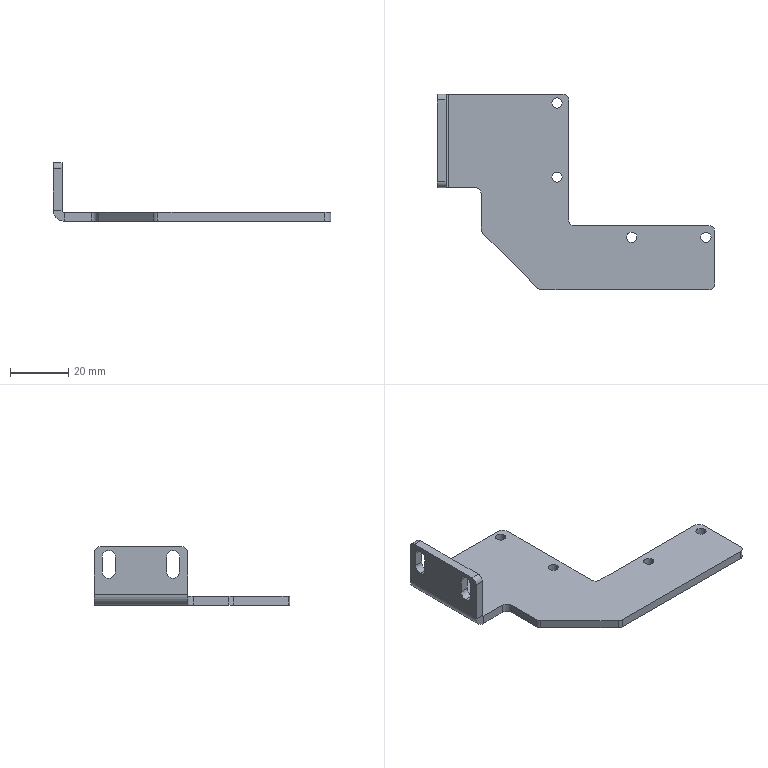Part | SolidWorks | features ICE 3, Chamfer 1, Cut 1, Fillet 1, FlatPattern 1, SMBaseFlange 1, SheetMetal 1 | 1 solid | 46 faces | box 95 x 67 x 20 mm | volume 11356 mm3 | cylinder 25 | plane 21 | commonest cylinder face diameters 4 x9 3.5 x8 4.5 x6 1.473 x1 7.473 x1
STEP:
#1=CARTESIAN_POINT('',(42.75,13.,-20.));
#2=VERTEX_POINT('',#1);
#3=CARTESIAN_POINT('',(39.25,13.,-20.));
#4=VERTEX_POINT('',#3);
#5=CARTESIAN_POINT('',(41.,13.,-20.));
#6=DIRECTION('',(0.,0.,-1.));
#7=DIRECTION('',(-1.,0.,0.));
#8=AXIS2_PLACEMENT_3D('',#5,#6,#7);
#9=CIRCLE('',#8,1.75);
#10=EDGE_CURVE('',#2,#4,#9,.T.);
#11=ORIENTED_EDGE('',*,*,#10,.T.);
#12=CARTESIAN_POINT('',(39.25,13.,-17.));
#13=VERTEX_POINT('',#12);
#14=CARTESIAN_POINT('',(39.25,13.,-27.));
#15=DIRECTION('',(0.,0.,1.));
#16=VECTOR('',#15,1000.);
#17=LINE('',#14,#16);
#18=EDGE_CURVE('',#4,#13,#17,.T.);
#19=ORIENTED_EDGE('',*,*,#18,.T.);
#20=CARTESIAN_POINT('',(42.75,13.,-17.));
#21=VERTEX_POINT('',#20);
#22=CARTESIAN_POINT('',(41.,13.,-17.));
#23=DIRECTION('',(0.,0.,1.));
#24=DIRECTION('',(1.,0.,0.));
#25=AXIS2_PLACEMENT_3D('',#22,#23,#24);
#26=CIRCLE('',#25,1.75);
#27=EDGE_CURVE('',#13,#21,#26,.T.);
#28=ORIENTED_EDGE('',*,*,#27,.T.);
#29=CARTESIAN_POINT('',(42.75,13.,-27.));
#30=DIRECTION('',(0.,0.,1.));
#31=VECTOR('',#30,1000.);
#32=LINE('',#29,#31);
#33=EDGE_CURVE('',#2,#21,#32,.T.);
#34=ORIENTED_EDGE('',*,*,#33,.F.);
#35=EDGE_LOOP('',(#11,#19,#28,#34));
#36=FACE_OUTER_BOUND('',#35,.T.);
#37=CARTESIAN_POINT('',(41.,13.,-27.));
#38=DIRECTION('',(0.,0.,1.));
#39=DIRECTION('',(1.,0.,0.));
#40=AXIS2_PLACEMENT_3D('',#37,#38,#39);
#41=CYLINDRICAL_SURFACE('',#40,1.75);
#42=ADVANCED_FACE('',(#36),#41,.F.);
#43=CARTESIAN_POINT('',(42.75,-12.4,-20.));
#44=VERTEX_POINT('',#43);
#45=CARTESIAN_POINT('',(39.25,-12.4,-20.));
#46=VERTEX_POINT('',#45);
#47=CARTESIAN_POINT('',(41.,-12.4,-20.));
#48=DIRECTION('',(0.,0.,-1.));
#49=DIRECTION('',(-1.,0.,0.));
#50=AXIS2_PLACEMENT_3D('',#47,#48,#49);
#51=CIRCLE('',#50,1.75);
#52=EDGE_CURVE('',#44,#46,#51,.T.);
#53=ORIENTED_EDGE('',*,*,#52,.T.);
#54=CARTESIAN_POINT('',(39.25,-12.4,-17.));
#55=VERTEX_POINT('',#54);
#56=CARTESIAN_POINT('',(39.25,-12.4,-27.));
#57=DIRECTION('',(0.,0.,1.));
#58=VECTOR('',#57,1000.);
#59=LINE('',#56,#58);
#60=EDGE_CURVE('',#46,#55,#59,.T.);
#61=ORIENTED_EDGE('',*,*,#60,.T.);
#62=CARTESIAN_POINT('',(42.75,-12.4,-17.));
#63=VERTEX_POINT('',#62);
#64=CARTESIAN_POINT('',(41.,-12.4,-17.));
#65=DIRECTION('',(0.,0.,1.));
#66=DIRECTION('',(1.,0.,0.));
#67=AXIS2_PLACEMENT_3D('',#64,#65,#66);
#68=CIRCLE('',#67,1.75);
#69=EDGE_CURVE('',#55,#63,#68,.T.);
#70=ORIENTED_EDGE('',*,*,#69,.T.);
#71=CARTESIAN_POINT('',(42.75,-12.4,-27.));
#72=DIRECTION('',(0.,0.,1.));
#73=VECTOR('',#72,1000.);
#74=LINE('',#71,#73);
#75=EDGE_CURVE('',#44,#63,#74,.T.);
#76=ORIENTED_EDGE('',*,*,#75,.F.);
#77=EDGE_LOOP('',(#53,#61,#70,#76));
#78=FACE_OUTER_BOUND('',#77,.T.);
#79=CARTESIAN_POINT('',(41.,-12.4,-27.));
#80=DIRECTION('',(0.,0.,1.));
#81=DIRECTION('',(1.,0.,0.));
#82=AXIS2_PLACEMENT_3D('',#79,#80,#81);
#83=CYLINDRICAL_SURFACE('',#82,1.75);
#84=ADVANCED_FACE('',(#78),#83,.F.);
#85=CARTESIAN_POINT('',(68.35,-33.,-20.));
#86=VERTEX_POINT('',#85);
#87=CARTESIAN_POINT('',(64.85,-33.,-20.));
#88=VERTEX_POINT('',#87);
#89=CARTESIAN_POINT('',(66.6,-33.,-20.));
#90=DIRECTION('',(0.,0.,-1.));
#91=DIRECTION('',(-1.,0.,0.));
#92=AXIS2_PLACEMENT_3D('',#89,#90,#91);
#93=CIRCLE('',#92,1.75);
#94=EDGE_CURVE('',#86,#88,#93,.T.);
#95=ORIENTED_EDGE('',*,*,#94,.T.);
#96=CARTESIAN_POINT('',(64.85,-33.,-17.));
#97=VERTEX_POINT('',#96);
#98=CARTESIAN_POINT('',(64.85,-33.,-27.));
#99=DIRECTION('',(0.,0.,1.));
#100=VECTOR('',#99,1000.);
#101=LINE('',#98,#100);
#102=EDGE_CURVE('',#88,#97,#101,.T.);
#103=ORIENTED_EDGE('',*,*,#102,.T.);
#104=CARTESIAN_POINT('',(68.35,-33.,-17.));
#105=VERTEX_POINT('',#104);
#106=CARTESIAN_POINT('',(66.6,-33.,-17.));
#107=DIRECTION('',(0.,0.,1.));
#108=DIRECTION('',(1.,0.,0.));
#109=AXIS2_PLACEMENT_3D('',#106,#107,#108);
#110=CIRCLE('',#109,1.75);
#111=EDGE_CURVE('',#97,#105,#110,.T.);
#112=ORIENTED_EDGE('',*,*,#111,.T.);
#113=CARTESIAN_POINT('',(68.35,-33.,-27.));
#114=DIRECTION('',(0.,0.,1.));
#115=VECTOR('',#114,1000.);
#116=LINE('',#113,#115);
#117=EDGE_CURVE('',#86,#105,#116,.T.);
#118=ORIENTED_EDGE('',*,*,#117,.F.);
#119=EDGE_LOOP('',(#95,#103,#112,#118));
#120=FACE_OUTER_BOUND('',#119,.T.);
#121=CARTESIAN_POINT('',(66.6,-33.,-27.));
#122=DIRECTION('',(0.,0.,1.));
#123=DIRECTION('',(1.,0.,0.));
#124=AXIS2_PLACEMENT_3D('',#121,#122,#123);
#125=CYLINDRICAL_SURFACE('',#124,1.75);
#126=ADVANCED_FACE('',(#120),#125,.F.);
#127=CARTESIAN_POINT('',(93.75,-33.,-20.));
#128=VERTEX_POINT('',#127);
#129=CARTESIAN_POINT('',(90.25,-33.,-20.));
#130=VERTEX_POINT('',#129);
#131=CARTESIAN_POINT('',(92.,-33.,-20.));
#132=DIRECTION('',(0.,0.,-1.));
#133=DIRECTION('',(-1.,0.,0.));
#134=AXIS2_PLACEMENT_3D('',#131,#132,#133);
#135=CIRCLE('',#134,1.75);
#136=EDGE_CURVE('',#128,#130,#135,.T.);
#137=ORIENTED_EDGE('',*,*,#136,.T.);
#138=CARTESIAN_POINT('',(90.25,-33.,-17.));
#139=VERTEX_POINT('',#138);
#140=CARTESIAN_POINT('',(90.25,-33.,-27.));
#141=DIRECTION('',(0.,0.,1.));
#142=VECTOR('',#141,1000.);
#143=LINE('',#140,#142);
#144=EDGE_CURVE('',#130,#139,#143,.T.);
#145=ORIENTED_EDGE('',*,*,#144,.T.);
#146=CARTESIAN_POINT('',(93.75,-33.,-17.));
#147=VERTEX_POINT('',#146);
#148=CARTESIAN_POINT('',(92.,-33.,-17.));
#149=DIRECTION('',(0.,0.,1.));
#150=DIRECTION('',(1.,0.,0.));
#151=AXIS2_PLACEMENT_3D('',#148,#149,#150);
#152=CIRCLE('',#151,1.75);
#153=EDGE_CURVE('',#139,#147,#152,.T.);
#154=ORIENTED_EDGE('',*,*,#153,.T.);
#155=CARTESIAN_POINT('',(93.75,-33.,-27.));
#156=DIRECTION('',(0.,0.,1.));
#157=VECTOR('',#156,1000.);
#158=LINE('',#155,#157);
#159=EDGE_CURVE('',#128,#147,#158,.T.);
#160=ORIENTED_EDGE('',*,*,#159,.F.);
#161=EDGE_LOOP('',(#137,#145,#154,#160));
#162=FACE_OUTER_BOUND('',#161,.T.);
#163=CARTESIAN_POINT('',(92.,-33.,-27.));
#164=DIRECTION('',(0.,0.,1.));
#165=DIRECTION('',(1.,0.,0.));
#166=AXIS2_PLACEMENT_3D('',#163,#164,#165);
#167=CYLINDRICAL_SURFACE('',#166,1.75);
#168=ADVANCED_FACE('',(#162),#167,.F.);
#169=CARTESIAN_POINT('',(0.,-11.,-10.75));
#170=VERTEX_POINT('',#169);
#171=CARTESIAN_POINT('',(0.,-8.75,-8.5));
#172=VERTEX_POINT('',#171);
#173=CARTESIAN_POINT('',(0.,-11.,-8.5));
#174=DIRECTION('',(1.,0.,0.));
#175=DIRECTION('',(0.,0.,-1.));
#176=AXIS2_PLACEMENT_3D('',#173,#174,#175);
#177=CIRCLE('',#176,2.25);
#178=EDGE_CURVE('',#170,#172,#177,.T.);
#179=ORIENTED_EDGE('',*,*,#178,.F.);
#180=CARTESIAN_POINT('',(3.,-11.,-10.75));
#181=VERTEX_POINT('',#180);
#182=CARTESIAN_POINT('',(0.,-11.,-10.75));
#183=DIRECTION('',(1.,0.,0.));
#184=VECTOR('',#183,1000.);
#185=LINE('',#182,#184);
#186=EDGE_CURVE('',#170,#181,#185,.T.);
#187=ORIENTED_EDGE('',*,*,#186,.T.);
#188=CARTESIAN_POINT('',(3.,-8.75,-8.5));
#189=VERTEX_POINT('',#188);
#190=CARTESIAN_POINT('',(3.,-11.,-8.5));
#191=DIRECTION('',(1.,0.,0.));
#192=DIRECTION('',(0.,0.,-1.));
#193=AXIS2_PLACEMENT_3D('',#190,#191,#192);
#194=CIRCLE('',#193,2.25);
#195=EDGE_CURVE('',#181,#189,#194,.T.);
#196=ORIENTED_EDGE('',*,*,#195,.T.);
#197=CARTESIAN_POINT('',(0.,-8.75,-8.5));
#198=DIRECTION('',(1.,0.,0.));
#199=VECTOR('',#198,1000.);
#200=LINE('',#197,#199);
#201=EDGE_CURVE('',#172,#189,#200,.T.);
#202=ORIENTED_EDGE('',*,*,#201,.F.);
#203=EDGE_LOOP('',(#179,#187,#196,#202));
#204=FACE_OUTER_BOUND('',#203,.T.);
#205=CARTESIAN_POINT('',(0.,-11.,-8.5));
#206=DIRECTION('',(1.,0.,0.));
#207=DIRECTION('',(0.,0.,-1.));
#208=AXIS2_PLACEMENT_3D('',#205,#206,#207);
#209=CYLINDRICAL_SURFACE('',#208,2.25);
#210=ADVANCED_FACE('',(#204),#209,.F.);
#211=CARTESIAN_POINT('',(0.,11.,-10.75));
#212=VERTEX_POINT('',#211);
#213=CARTESIAN_POINT('',(0.,13.25,-8.5));
#214=VERTEX_POINT('',#213);
#215=CARTESIAN_POINT('',(0.,11.,-8.5));
#216=DIRECTION('',(1.,0.,0.));
#217=DIRECTION('',(0.,0.,1.));
#218=AXIS2_PLACEMENT_3D('',#215,#216,#217);
#219=CIRCLE('',#218,2.25);
#220=EDGE_CURVE('',#212,#214,#219,.T.);
#221=ORIENTED_EDGE('',*,*,#220,.F.);
#222=CARTESIAN_POINT('',(3.,11.,-10.75));
#223=VERTEX_POINT('',#222);
#224=CARTESIAN_POINT('',(0.,11.,-10.75));
#225=DIRECTION('',(1.,0.,0.));
#226=VECTOR('',#225,1000.);
#227=LINE('',#224,#226);
#228=EDGE_CURVE('',#212,#223,#227,.T.);
#229=ORIENTED_EDGE('',*,*,#228,.T.);
#230=CARTESIAN_POINT('',(3.,13.25,-8.5));
#231=VERTEX_POINT('',#230);
#232=CARTESIAN_POINT('',(3.,11.,-8.5));
#233=DIRECTION('',(1.,0.,0.));
#234=DIRECTION('',(0.,0.,1.));
#235=AXIS2_PLACEMENT_3D('',#232,#233,#234);
#236=CIRCLE('',#235,2.25);
#237=EDGE_CURVE('',#223,#231,#236,.T.);
#238=ORIENTED_EDGE('',*,*,#237,.T.);
#239=CARTESIAN_POINT('',(0.,13.25,-8.5));
#240=DIRECTION('',(1.,0.,0.));
#241=VECTOR('',#240,1000.);
#242=LINE('',#239,#241);
#243=EDGE_CURVE('',#214,#231,#242,.T.);
#244=ORIENTED_EDGE('',*,*,#243,.F.);
#245=EDGE_LOOP('',(#221,#229,#238,#244));
#246=FACE_OUTER_BOUND('',#245,.T.);
#247=CARTESIAN_POINT('',(0.,11.,-8.5));
#248=DIRECTION('',(1.,0.,0.));
#249=DIRECTION('',(0.,0.,-1.));
#250=AXIS2_PLACEMENT_3D('',#247,#248,#249);
#251=CYLINDRICAL_SURFACE('',#250,2.25);
#252=ADVANCED_FACE('',(#246),#251,.F.);
#253=CARTESIAN_POINT('',(3.737,-16.,-20.));
#254=VERTEX_POINT('',#253);
#255=CARTESIAN_POINT('',(13.,-16.,-20.));
#256=VERTEX_POINT('',#255);
#257=CARTESIAN_POINT('',(0.,-16.,-20.));
#258=DIRECTION('',(1.,0.,0.));
#259=VECTOR('',#258,1000.);
#260=LINE('',#257,#259);
#261=EDGE_CURVE('',#254,#256,#260,.T.);
#262=ORIENTED_EDGE('',*,*,#261,.T.);
#263=CARTESIAN_POINT('',(13.,-16.,-17.));
#264=VERTEX_POINT('',#263);
#265=CARTESIAN_POINT('',(13.,-16.,-17.));
#266=DIRECTION('',(0.,0.,1.));
#267=VECTOR('',#266,1000.);
#268=LINE('',#265,#267);
#269=EDGE_CURVE('',#256,#264,#268,.T.);
#270=ORIENTED_EDGE('',*,*,#269,.T.);
#271=CARTESIAN_POINT('',(3.737,-16.,-17.));
#272=VERTEX_POINT('',#271);
#273=CARTESIAN_POINT('',(0.,-16.,-17.));
#274=DIRECTION('',(1.,0.,0.));
#275=VECTOR('',#274,1000.);
#276=LINE('',#273,#275);
#277=EDGE_CURVE('',#272,#264,#276,.T.);
#278=ORIENTED_EDGE('',*,*,#277,.F.);
#279=CARTESIAN_POINT('',(3.737,-16.,-17.));
#280=DIRECTION('',(0.,0.,-1.));
#281=VECTOR('',#280,1000.);
#282=LINE('',#279,#281);
#283=EDGE_CURVE('',#272,#254,#282,.T.);
#284=ORIENTED_EDGE('',*,*,#283,.T.);
#285=EDGE_LOOP('',(#262,#270,#278,#284));
#286=FACE_OUTER_BOUND('',#285,.T.);
#287=CARTESIAN_POINT('',(3.737,-16.,-16.263));
#288=DIRECTION('',(0.,1.,0.));
#289=DIRECTION('',(1.,0.,0.));
#290=AXIS2_PLACEMENT_3D('',#287,#288,#289);
#291=PLANE('',#290);
#292=ADVANCED_FACE('',(#286),#291,.F.);
#293=CARTESIAN_POINT('',(3.737,16.,-20.));
#294=VERTEX_POINT('',#293);
#295=CARTESIAN_POINT('',(3.737,16.,-17.));
#296=VERTEX_POINT('',#295);
#297=CARTESIAN_POINT('',(3.737,16.,-20.));
#298=DIRECTION('',(0.,0.,1.));
#299=VECTOR('',#298,1000.);
#300=LINE('',#297,#299);
#301=EDGE_CURVE('',#294,#296,#300,.T.);
#302=ORIENTED_EDGE('',*,*,#301,.F.);
#303=CARTESIAN_POINT('',(0.,16.,-16.263));
#304=VERTEX_POINT('',#303);
#305=CARTESIAN_POINT('',(3.737,16.,-16.263));
#306=DIRECTION('',(0.,-1.,0.));
#307=DIRECTION('',(0.,0.,1.));
#308=AXIS2_PLACEMENT_3D('',#305,#306,#307);
#309=CIRCLE('',#308,3.737);
#310=EDGE_CURVE('',#304,#294,#309,.T.);
#311=ORIENTED_EDGE('',*,*,#310,.F.);
#312=CARTESIAN_POINT('',(3.,16.,-16.263));
#313=VERTEX_POINT('',#312);
#314=CARTESIAN_POINT('',(3.,16.,-16.263));
#315=DIRECTION('',(-1.,0.,0.));
#316=VECTOR('',#315,1000.);
#317=LINE('',#314,#316);
#318=EDGE_CURVE('',#313,#304,#317,.T.);
#319=ORIENTED_EDGE('',*,*,#318,.F.);
#320=CARTESIAN_POINT('',(3.737,16.,-16.263));
#321=DIRECTION('',(0.,-1.,0.));
#322=DIRECTION('',(1.,0.,0.));
#323=AXIS2_PLACEMENT_3D('',#320,#321,#322);
#324=CIRCLE('',#323,0.7366);
#325=EDGE_CURVE('',#313,#296,#324,.T.);
#326=ORIENTED_EDGE('',*,*,#325,.T.);
#327=EDGE_LOOP('',(#302,#311,#319,#326));
#328=FACE_OUTER_BOUND('',#327,.T.);
#329=CARTESIAN_POINT('',(3.737,16.,-20.));
#330=DIRECTION('',(0.,1.,0.));
#331=DIRECTION('',(0.,0.,1.));
#332=AXIS2_PLACEMENT_3D('',#329,#330,#331);
#333=PLANE('',#332);
#334=ADVANCED_FACE('',(#328),#333,.T.);
#335=CARTESIAN_POINT('',(43.,16.,-17.));
#336=VERTEX_POINT('',#335);
#337=CARTESIAN_POINT('',(0.,16.,-17.));
#338=DIRECTION('',(1.,0.,0.));
#339=VECTOR('',#338,1000.);
#340=LINE('',#337,#339);
#341=EDGE_CURVE('',#296,#336,#340,.T.);
#342=ORIENTED_EDGE('',*,*,#341,.T.);
#343=CARTESIAN_POINT('',(43.,16.,-20.));
#344=VERTEX_POINT('',#343);
#345=CARTESIAN_POINT('',(43.,16.,-16.263));
#346=DIRECTION('',(0.,0.,-1.));
#347=VECTOR('',#346,1000.);
#348=LINE('',#345,#347);
#349=EDGE_CURVE('',#336,#344,#348,.T.);
#350=ORIENTED_EDGE('',*,*,#349,.T.);
#351=CARTESIAN_POINT('',(0.,16.,-20.));
#352=DIRECTION('',(1.,0.,0.));
#353=VECTOR('',#352,1000.);
#354=LINE('',#351,#353);
#355=EDGE_CURVE('',#294,#344,#354,.T.);
#356=ORIENTED_EDGE('',*,*,#355,.F.);
#357=ORIENTED_EDGE('',*,*,#301,.T.);
#358=EDGE_LOOP('',(#342,#350,#356,#357));
#359=FACE_OUTER_BOUND('',#358,.T.);
#360=CARTESIAN_POINT('',(3.,16.,-16.263));
#361=DIRECTION('',(0.,1.,0.));
#362=DIRECTION('',(0.,0.,1.));
#363=AXIS2_PLACEMENT_3D('',#360,#361,#362);
#364=PLANE('',#363);
#365=ADVANCED_FACE('',(#359),#364,.T.);
#366=CARTESIAN_POINT('',(0.,-16.,-16.263));
#367=VERTEX_POINT('',#366);
#368=CARTESIAN_POINT('',(3.,-16.,-16.263));
#369=VERTEX_POINT('',#368);
#370=CARTESIAN_POINT('',(0.,-16.,-16.263));
#371=DIRECTION('',(1.,0.,0.));
#372=VECTOR('',#371,1000.);
#373=LINE('',#370,#372);
#374=EDGE_CURVE('',#367,#369,#373,.T.);
#375=ORIENTED_EDGE('',*,*,#374,.F.);
#376=CARTESIAN_POINT('',(3.737,-16.,-16.263));
#377=DIRECTION('',(0.,-1.,0.));
#378=DIRECTION('',(0.,0.,1.));
#379=AXIS2_PLACEMENT_3D('',#376,#377,#378);
#380=CIRCLE('',#379,3.737);
#381=EDGE_CURVE('',#367,#254,#380,.T.);
#382=ORIENTED_EDGE('',*,*,#381,.T.);
#383=ORIENTED_EDGE('',*,*,#283,.F.);
#384=CARTESIAN_POINT('',(3.737,-16.,-16.263));
#385=DIRECTION('',(0.,-1.,0.));
#386=DIRECTION('',(1.,0.,0.));
#387=AXIS2_PLACEMENT_3D('',#384,#385,#386);
#388=CIRCLE('',#387,0.7366);
#389=EDGE_CURVE('',#369,#272,#388,.T.);
#390=ORIENTED_EDGE('',*,*,#389,.F.);
#391=EDGE_LOOP('',(#375,#382,#383,#390));
#392=FACE_OUTER_BOUND('',#391,.T.);
#393=CARTESIAN_POINT('',(0.,-16.,-16.263));
#394=DIRECTION('',(0.,-1.,0.));
#395=DIRECTION('',(0.,0.,-1.));
#396=AXIS2_PLACEMENT_3D('',#393,#394,#395);
#397=PLANE('',#396);
#398=ADVANCED_FACE('',(#392),#397,.T.);
#399=CARTESIAN_POINT('',(3.,-16.,-2.));
#400=VERTEX_POINT('',#399);
#401=CARTESIAN_POINT('',(3.,-16.,0.));
#402=DIRECTION('',(0.,0.,-1.));
#403=VECTOR('',#402,1000.);
#404=LINE('',#401,#403);
#405=EDGE_CURVE('',#400,#369,#404,.T.);
#406=ORIENTED_EDGE('',*,*,#405,.F.);
#407=CARTESIAN_POINT('',(0.,-16.,-2.));
#408=VERTEX_POINT('',#407);
#409=CARTESIAN_POINT('',(3.737,-16.,-2.));
#410=DIRECTION('',(-1.,0.,0.));
#411=VECTOR('',#410,1000.);
#412=LINE('',#409,#411);
#413=EDGE_CURVE('',#400,#408,#412,.T.);
#414=ORIENTED_EDGE('',*,*,#413,.T.);
#415=CARTESIAN_POINT('',(0.,-16.,0.));
#416=DIRECTION('',(0.,0.,-1.));
#417=VECTOR('',#416,1000.);
#418=LINE('',#415,#417);
#419=EDGE_CURVE('',#408,#367,#418,.T.);
#420=ORIENTED_EDGE('',*,*,#419,.T.);
#421=ORIENTED_EDGE('',*,*,#374,.T.);
#422=EDGE_LOOP('',(#406,#414,#420,#421));
#423=FACE_OUTER_BOUND('',#422,.T.);
#424=CARTESIAN_POINT('',(3.737,-16.,-17.));
#425=DIRECTION('',(0.,-1.,0.));
#426=DIRECTION('',(0.,0.,-1.));
#427=AXIS2_PLACEMENT_3D('',#424,#425,#426);
#428=PLANE('',#427);
#429=ADVANCED_FACE('',(#423),#428,.T.);
#430=CARTESIAN_POINT('',(41.,13.,-17.));
#431=DIRECTION('',(0.,0.,1.));
#432=DIRECTION('',(1.,0.,0.));
#433=AXIS2_PLACEMENT_3D('',#430,#431,#432);
#434=CIRCLE('',#433,1.75);
#435=EDGE_CURVE('',#21,#13,#434,.T.);
#436=ORIENTED_EDGE('',*,*,#435,.F.);
#437=ORIENTED_EDGE('',*,*,#27,.F.);
#438=EDGE_LOOP('',(#436,#437));
#439=FACE_BOUND('',#438,.T.);
#440=CARTESIAN_POINT('',(41.,-12.4,-17.));
#441=DIRECTION('',(0.,0.,1.));
#442=DIRECTION('',(1.,0.,0.));
#443=AXIS2_PLACEMENT_3D('',#440,#441,#442);
#444=CIRCLE('',#443,1.75);
#445=EDGE_CURVE('',#63,#55,#444,.T.);
#446=ORIENTED_EDGE('',*,*,#445,.F.);
#447=ORIENTED_EDGE('',*,*,#69,.F.);
#448=EDGE_LOOP('',(#446,#447));
#449=FACE_BOUND('',#448,.T.);
#450=CARTESIAN_POINT('',(66.6,-33.,-17.));
#451=DIRECTION('',(0.,0.,1.));
#452=DIRECTION('',(1.,0.,0.));
#453=AXIS2_PLACEMENT_3D('',#450,#451,#452);
#454=CIRCLE('',#453,1.75);
#455=EDGE_CURVE('',#105,#97,#454,.T.);
#456=ORIENTED_EDGE('',*,*,#455,.F.);
#457=ORIENTED_EDGE('',*,*,#111,.F.);
#458=EDGE_LOOP('',(#456,#457));
#459=FACE_BOUND('',#458,.T.);
#460=CARTESIAN_POINT('',(92.,-33.,-17.));
#461=DIRECTION('',(0.,0.,1.));
#462=DIRECTION('',(1.,0.,0.));
#463=AXIS2_PLACEMENT_3D('',#460,#461,#462);
#464=CIRCLE('',#463,1.75);
#465=EDGE_CURVE('',#147,#139,#464,.T.);
#466=ORIENTED_EDGE('',*,*,#465,.F.);
#467=ORIENTED_EDGE('',*,*,#153,.F.);
#468=EDGE_LOOP('',(#466,#467));
#469=FACE_BOUND('',#468,.T.);
#470=CARTESIAN_POINT('',(15.586,-31.586,-17.));
#471=VERTEX_POINT('',#470);
#472=CARTESIAN_POINT('',(34.414,-50.414,-17.));
#473=VERTEX_POINT('',#472);
#474=CARTESIAN_POINT('',(35.,-51.,-17.));
#475=DIRECTION('',(0.7071,-0.7071,0.));
#476=VECTOR('',#475,1000.);
#477=LINE('',#474,#476);
#478=EDGE_CURVE('',#471,#473,#477,.T.);
#479=ORIENTED_EDGE('',*,*,#478,.T.);
#480=CARTESIAN_POINT('',(35.828,-51.,-17.));
#481=VERTEX_POINT('',#480);
#482=CARTESIAN_POINT('',(35.828,-49.,-17.));
#483=DIRECTION('',(0.,0.,1.));
#484=DIRECTION('',(-1.,0.,0.));
#485=AXIS2_PLACEMENT_3D('',#482,#483,#484);
#486=CIRCLE('',#485,2.);
#487=EDGE_CURVE('',#473,#481,#486,.T.);
#488=ORIENTED_EDGE('',*,*,#487,.T.);
#489=CARTESIAN_POINT('',(93.,-51.,-17.));
#490=VERTEX_POINT('',#489);
#491=CARTESIAN_POINT('',(45.,-51.,-17.));
#492=DIRECTION('',(-1.,0.,0.));
#493=VECTOR('',#492,1000.);
#494=LINE('',#491,#493);
#495=EDGE_CURVE('',#490,#481,#494,.T.);
#496=ORIENTED_EDGE('',*,*,#495,.F.);
#497=CARTESIAN_POINT('',(95.,-49.,-17.));
#498=VERTEX_POINT('',#497);
#499=CARTESIAN_POINT('',(93.,-49.,-17.));
#500=DIRECTION('',(0.,0.,1.));
#501=DIRECTION('',(-1.,0.,0.));
#502=AXIS2_PLACEMENT_3D('',#499,#500,#501);
#503=CIRCLE('',#502,2.);
#504=EDGE_CURVE('',#490,#498,#503,.T.);
#505=ORIENTED_EDGE('',*,*,#504,.T.);
#506=CARTESIAN_POINT('',(95.,-31.,-17.));
#507=VERTEX_POINT('',#506);
#508=CARTESIAN_POINT('',(95.,-51.,-17.));
#509=DIRECTION('',(0.,-1.,0.));
#510=VECTOR('',#509,1000.);
#511=LINE('',#508,#510);
#512=EDGE_CURVE('',#507,#498,#511,.T.);
#513=ORIENTED_EDGE('',*,*,#512,.F.);
#514=CARTESIAN_POINT('',(93.,-29.,-17.));
#515=VERTEX_POINT('',#514);
#516=CARTESIAN_POINT('',(93.,-31.,-17.));
#517=DIRECTION('',(0.,0.,1.));
#518=DIRECTION('',(-1.,0.,0.));
#519=AXIS2_PLACEMENT_3D('',#516,#517,#518);
#520=CIRCLE('',#519,2.);
#521=EDGE_CURVE('',#507,#515,#520,.T.);
#522=ORIENTED_EDGE('',*,*,#521,.T.);
#523=CARTESIAN_POINT('',(47.,-29.,-17.));
#524=VERTEX_POINT('',#523);
#525=CARTESIAN_POINT('',(95.,-29.,-17.));
#526=DIRECTION('',(-1.,0.,0.));
#527=VECTOR('',#526,1000.);
#528=LINE('',#525,#527);
#529=EDGE_CURVE('',#515,#524,#528,.T.);
#530=ORIENTED_EDGE('',*,*,#529,.T.);
#531=CARTESIAN_POINT('',(45.,-27.,-17.));
#532=VERTEX_POINT('',#531);
#533=CARTESIAN_POINT('',(47.,-27.,-17.));
#534=DIRECTION('',(0.,0.,-1.));
#535=DIRECTION('',(-1.,0.,0.));
#536=AXIS2_PLACEMENT_3D('',#533,#534,#535);
#537=CIRCLE('',#536,2.);
#538=EDGE_CURVE('',#524,#532,#537,.T.);
#539=ORIENTED_EDGE('',*,*,#538,.T.);
#540=CARTESIAN_POINT('',(45.,14.,-17.));
#541=VERTEX_POINT('',#540);
#542=CARTESIAN_POINT('',(45.,16.,-17.));
#543=DIRECTION('',(0.,-1.,0.));
#544=VECTOR('',#543,1000.);
#545=LINE('',#542,#544);
#546=EDGE_CURVE('',#541,#532,#545,.T.);
#547=ORIENTED_EDGE('',*,*,#546,.F.);
#548=CARTESIAN_POINT('',(43.,14.,-17.));
#549=DIRECTION('',(0.,0.,1.));
#550=DIRECTION('',(-1.,0.,0.));
#551=AXIS2_PLACEMENT_3D('',#548,#549,#550);
#552=CIRCLE('',#551,2.);
#553=EDGE_CURVE('',#541,#336,#552,.T.);
#554=ORIENTED_EDGE('',*,*,#553,.T.);
#555=ORIENTED_EDGE('',*,*,#341,.F.);
#556=CARTESIAN_POINT('',(3.737,16.,-17.));
#557=DIRECTION('',(0.,-1.,0.));
#558=VECTOR('',#557,1000.);
#559=LINE('',#556,#558);
#560=EDGE_CURVE('',#296,#272,#559,.T.);
#561=ORIENTED_EDGE('',*,*,#560,.T.);
#562=ORIENTED_EDGE('',*,*,#277,.T.);
#563=CARTESIAN_POINT('',(15.,-18.,-17.));
#564=VERTEX_POINT('',#563);
#565=CARTESIAN_POINT('',(13.,-18.,-17.));
#566=DIRECTION('',(0.,0.,-1.));
#567=DIRECTION('',(-1.,0.,0.));
#568=AXIS2_PLACEMENT_3D('',#565,#566,#567);
#569=CIRCLE('',#568,2.);
#570=EDGE_CURVE('',#264,#564,#569,.T.);
#571=ORIENTED_EDGE('',*,*,#570,.T.);
#572=CARTESIAN_POINT('',(15.,-30.172,-17.));
#573=VERTEX_POINT('',#572);
#574=CARTESIAN_POINT('',(15.,-51.,-17.));
#575=DIRECTION('',(0.,1.,0.));
#576=VECTOR('',#575,1000.);
#577=LINE('',#574,#576);
#578=EDGE_CURVE('',#573,#564,#577,.T.);
#579=ORIENTED_EDGE('',*,*,#578,.F.);
#580=CARTESIAN_POINT('',(17.,-30.172,-17.));
#581=DIRECTION('',(0.,0.,1.));
#582=DIRECTION('',(-1.,0.,0.));
#583=AXIS2_PLACEMENT_3D('',#580,#581,#582);
#584=CIRCLE('',#583,2.);
#585=EDGE_CURVE('',#573,#471,#584,.T.);
#586=ORIENTED_EDGE('',*,*,#585,.T.);
#587=EDGE_LOOP('',(#479,#488,#496,#505,#513,#522,#530,#539,#547,#554,#555,#561,#562,#571,#579,#586));
#588=FACE_OUTER_BOUND('',#587,.T.);
#589=CARTESIAN_POINT('',(0.,16.,-17.));
#590=DIRECTION('',(0.,0.,-1.));
#591=DIRECTION('',(-1.,0.,0.));
#592=AXIS2_PLACEMENT_3D('',#589,#590,#591);
#593=PLANE('',#592);
#594=ADVANCED_FACE('',(#439,#449,#459,#469,#588),#593,.F.);
#595=ORIENTED_EDGE('',*,*,#546,.T.);
#596=CARTESIAN_POINT('',(45.,-27.,-20.));
#597=VERTEX_POINT('',#596);
#598=CARTESIAN_POINT('',(45.,-27.,-20.));
#599=DIRECTION('',(0.,0.,-1.));
#600=VECTOR('',#599,1000.);
#601=LINE('',#598,#600);
#602=EDGE_CURVE('',#532,#597,#601,.T.);
#603=ORIENTED_EDGE('',*,*,#602,.T.);
#604=CARTESIAN_POINT('',(45.,14.,-20.));
#605=VERTEX_POINT('',#604);
#606=CARTESIAN_POINT('',(45.,16.,-20.));
#607=DIRECTION('',(0.,-1.,0.));
#608=VECTOR('',#607,1000.);
#609=LINE('',#606,#608);
#610=EDGE_CURVE('',#605,#597,#609,.T.);
#611=ORIENTED_EDGE('',*,*,#610,.F.);
#612=CARTESIAN_POINT('',(45.,14.,-20.));
#613=DIRECTION('',(0.,0.,1.));
#614=VECTOR('',#613,1000.);
#615=LINE('',#612,#614);
#616=EDGE_CURVE('',#605,#541,#615,.T.);
#617=ORIENTED_EDGE('',*,*,#616,.T.);
#618=EDGE_LOOP('',(#595,#603,#611,#617));
#619=FACE_OUTER_BOUND('',#618,.T.);
#620=CARTESIAN_POINT('',(45.,16.,-20.));
#621=DIRECTION('',(1.,0.,0.));
#622=DIRECTION('',(0.,0.,-1.));
#623=AXIS2_PLACEMENT_3D('',#620,#621,#622);
#624=PLANE('',#623);
#625=ADVANCED_FACE('',(#619),#624,.T.);
#626=ORIENTED_EDGE('',*,*,#10,.F.);
#627=CARTESIAN_POINT('',(41.,13.,-20.));
#628=DIRECTION('',(0.,0.,-1.));
#629=DIRECTION('',(-1.,0.,0.));
#630=AXIS2_PLACEMENT_3D('',#627,#628,#629);
#631=CIRCLE('',#630,1.75);
#632=EDGE_CURVE('',#4,#2,#631,.T.);
#633=ORIENTED_EDGE('',*,*,#632,.F.);
#634=EDGE_LOOP('',(#626,#633));
#635=FACE_BOUND('',#634,.T.);
#636=ORIENTED_EDGE('',*,*,#52,.F.);
#637=CARTESIAN_POINT('',(41.,-12.4,-20.));
#638=DIRECTION('',(0.,0.,-1.));
#639=DIRECTION('',(-1.,0.,0.));
#640=AXIS2_PLACEMENT_3D('',#637,#638,#639);
#641=CIRCLE('',#640,1.75);
#642=EDGE_CURVE('',#46,#44,#641,.T.);
#643=ORIENTED_EDGE('',*,*,#642,.F.);
#644=EDGE_LOOP('',(#636,#643));
#645=FACE_BOUND('',#644,.T.);
#646=ORIENTED_EDGE('',*,*,#94,.F.);
#647=CARTESIAN_POINT('',(66.6,-33.,-20.));
#648=DIRECTION('',(0.,0.,-1.));
#649=DIRECTION('',(-1.,0.,0.));
#650=AXIS2_PLACEMENT_3D('',#647,#648,#649);
#651=CIRCLE('',#650,1.75);
#652=EDGE_CURVE('',#88,#86,#651,.T.);
#653=ORIENTED_EDGE('',*,*,#652,.F.);
#654=EDGE_LOOP('',(#646,#653));
#655=FACE_BOUND('',#654,.T.);
#656=ORIENTED_EDGE('',*,*,#136,.F.);
#657=CARTESIAN_POINT('',(92.,-33.,-20.));
#658=DIRECTION('',(0.,0.,-1.));
#659=DIRECTION('',(-1.,0.,0.));
#660=AXIS2_PLACEMENT_3D('',#657,#658,#659);
#661=CIRCLE('',#660,1.75);
#662=EDGE_CURVE('',#130,#128,#661,.T.);
#663=ORIENTED_EDGE('',*,*,#662,.F.);
#664=EDGE_LOOP('',(#656,#663));
#665=FACE_BOUND('',#664,.T.);
#666=CARTESIAN_POINT('',(35.828,-51.,-20.));
#667=VERTEX_POINT('',#666);
#668=CARTESIAN_POINT('',(93.,-51.,-20.));
#669=VERTEX_POINT('',#668);
#670=CARTESIAN_POINT('',(45.,-51.,-20.));
#671=DIRECTION('',(1.,0.,0.));
#672=VECTOR('',#671,1000.);
#673=LINE('',#670,#672);
#674=EDGE_CURVE('',#667,#669,#673,.T.);
#675=ORIENTED_EDGE('',*,*,#674,.F.);
#676=CARTESIAN_POINT('',(34.414,-50.414,-20.));
#677=VERTEX_POINT('',#676);
#678=CARTESIAN_POINT('',(35.828,-49.,-20.));
#679=DIRECTION('',(0.,0.,-1.));
#680=DIRECTION('',(-1.,0.,0.));
#681=AXIS2_PLACEMENT_3D('',#678,#679,#680);
#682=CIRCLE('',#681,2.);
#683=EDGE_CURVE('',#667,#677,#682,.T.);
#684=ORIENTED_EDGE('',*,*,#683,.T.);
#685=CARTESIAN_POINT('',(15.586,-31.586,-20.));
#686=VERTEX_POINT('',#685);
#687=CARTESIAN_POINT('',(-16.,0.,-20.));
#688=DIRECTION('',(-0.7071,0.7071,0.));
#689=VECTOR('',#688,1000.);
#690=LINE('',#687,#689);
#691=EDGE_CURVE('',#677,#686,#690,.T.);
#692=ORIENTED_EDGE('',*,*,#691,.T.);
#693=CARTESIAN_POINT('',(15.,-30.172,-20.));
#694=VERTEX_POINT('',#693);
#695=CARTESIAN_POINT('',(17.,-30.172,-20.));
#696=DIRECTION('',(0.,0.,-1.));
#697=DIRECTION('',(-1.,0.,0.));
#698=AXIS2_PLACEMENT_3D('',#695,#696,#697);
#699=CIRCLE('',#698,2.);
#700=EDGE_CURVE('',#686,#694,#699,.T.);
#701=ORIENTED_EDGE('',*,*,#700,.T.);
#702=CARTESIAN_POINT('',(15.,-18.,-20.));
#703=VERTEX_POINT('',#702);
#704=CARTESIAN_POINT('',(15.,-51.,-20.));
#705=DIRECTION('',(0.,1.,0.));
#706=VECTOR('',#705,1000.);
#707=LINE('',#704,#706);
#708=EDGE_CURVE('',#694,#703,#707,.T.);
#709=ORIENTED_EDGE('',*,*,#708,.T.);
#710=CARTESIAN_POINT('',(13.,-18.,-20.));
#711=DIRECTION('',(0.,0.,1.));
#712=DIRECTION('',(-1.,0.,0.));
#713=AXIS2_PLACEMENT_3D('',#710,#711,#712);
#714=CIRCLE('',#713,2.);
#715=EDGE_CURVE('',#703,#256,#714,.T.);
#716=ORIENTED_EDGE('',*,*,#715,.T.);
#717=ORIENTED_EDGE('',*,*,#261,.F.);
#718=CARTESIAN_POINT('',(3.737,16.,-20.));
#719=DIRECTION('',(0.,-1.,0.));
#720=VECTOR('',#719,1000.);
#721=LINE('',#718,#720);
#722=EDGE_CURVE('',#294,#254,#721,.T.);
#723=ORIENTED_EDGE('',*,*,#722,.F.);
#724=ORIENTED_EDGE('',*,*,#355,.T.);
#725=CARTESIAN_POINT('',(43.,14.,-20.));
#726=DIRECTION('',(0.,0.,-1.));
#727=DIRECTION('',(-1.,0.,0.));
#728=AXIS2_PLACEMENT_3D('',#725,#726,#727);
#729=CIRCLE('',#728,2.);
#730=EDGE_CURVE('',#344,#605,#729,.T.);
#731=ORIENTED_EDGE('',*,*,#730,.T.);
#732=ORIENTED_EDGE('',*,*,#610,.T.);
#733=CARTESIAN_POINT('',(47.,-29.,-20.));
#734=VERTEX_POINT('',#733);
#735=CARTESIAN_POINT('',(47.,-27.,-20.));
#736=DIRECTION('',(0.,0.,1.));
#737=DIRECTION('',(-1.,0.,0.));
#738=AXIS2_PLACEMENT_3D('',#735,#736,#737);
#739=CIRCLE('',#738,2.);
#740=EDGE_CURVE('',#597,#734,#739,.T.);
#741=ORIENTED_EDGE('',*,*,#740,.T.);
#742=CARTESIAN_POINT('',(93.,-29.,-20.));
#743=VERTEX_POINT('',#742);
#744=CARTESIAN_POINT('',(95.,-29.,-20.));
#745=DIRECTION('',(-1.,0.,0.));
#746=VECTOR('',#745,1000.);
#747=LINE('',#744,#746);
#748=EDGE_CURVE('',#743,#734,#747,.T.);
#749=ORIENTED_EDGE('',*,*,#748,.F.);
#750=CARTESIAN_POINT('',(95.,-31.,-20.));
#751=VERTEX_POINT('',#750);
#752=CARTESIAN_POINT('',(93.,-31.,-20.));
#753=DIRECTION('',(0.,0.,-1.));
#754=DIRECTION('',(-1.,0.,0.));
#755=AXIS2_PLACEMENT_3D('',#752,#753,#754);
#756=CIRCLE('',#755,2.);
#757=EDGE_CURVE('',#743,#751,#756,.T.);
#758=ORIENTED_EDGE('',*,*,#757,.T.);
#759=CARTESIAN_POINT('',(95.,-49.,-20.));
#760=VERTEX_POINT('',#759);
#761=CARTESIAN_POINT('',(95.,-51.,-20.));
#762=DIRECTION('',(0.,1.,0.));
#763=VECTOR('',#762,1000.);
#764=LINE('',#761,#763);
#765=EDGE_CURVE('',#760,#751,#764,.T.);
#766=ORIENTED_EDGE('',*,*,#765,.F.);
#767=CARTESIAN_POINT('',(93.,-49.,-20.));
#768=DIRECTION('',(0.,0.,-1.));
#769=DIRECTION('',(-1.,0.,0.));
#770=AXIS2_PLACEMENT_3D('',#767,#768,#769);
#771=CIRCLE('',#770,2.);
#772=EDGE_CURVE('',#760,#669,#771,.T.);
#773=ORIENTED_EDGE('',*,*,#772,.T.);
#774=EDGE_LOOP('',(#675,#684,#692,#701,#709,#716,#717,#723,#724,#731,#732,#741,#749,#758,#766,#773));
#775=FACE_OUTER_BOUND('',#774,.T.);
#776=CARTESIAN_POINT('',(0.,16.,-20.));
#777=DIRECTION('',(0.,0.,-1.));
#778=DIRECTION('',(-1.,0.,0.));
#779=AXIS2_PLACEMENT_3D('',#776,#777,#778);
#780=PLANE('',#779);
#781=ADVANCED_FACE('',(#635,#645,#655,#665,#775),#780,.T.);
#782=ORIENTED_EDGE('',*,*,#381,.F.);
#783=CARTESIAN_POINT('',(0.,16.,-16.263));
#784=DIRECTION('',(0.,-1.,0.));
#785=VECTOR('',#784,1000.);
#786=LINE('',#783,#785);
#787=EDGE_CURVE('',#304,#367,#786,.T.);
#788=ORIENTED_EDGE('',*,*,#787,.F.);
#789=ORIENTED_EDGE('',*,*,#310,.T.);
#790=ORIENTED_EDGE('',*,*,#722,.T.);
#791=EDGE_LOOP('',(#782,#788,#789,#790));
#792=FACE_OUTER_BOUND('',#791,.T.);
#793=CARTESIAN_POINT('',(3.737,16.,-16.263));
#794=DIRECTION('',(0.,-1.,0.));
#795=DIRECTION('',(0.,0.,-1.));
#796=AXIS2_PLACEMENT_3D('',#793,#794,#795);
#797=CYLINDRICAL_SURFACE('',#796,3.737);
#798=ADVANCED_FACE('',(#792),#797,.T.);
#799=CARTESIAN_POINT('',(0.,-8.75,-3.5));
#800=VERTEX_POINT('',#799);
#801=CARTESIAN_POINT('',(0.,-13.25,-3.5));
#802=VERTEX_POINT('',#801);
#803=CARTESIAN_POINT('',(0.,-11.,-3.5));
#804=DIRECTION('',(1.,0.,0.));
#805=DIRECTION('',(0.,0.,-1.));
#806=AXIS2_PLACEMENT_3D('',#803,#804,#805);
#807=CIRCLE('',#806,2.25);
#808=EDGE_CURVE('',#800,#802,#807,.T.);
#809=ORIENTED_EDGE('',*,*,#808,.T.);
#810=CARTESIAN_POINT('',(0.,-13.25,-8.5));
#811=VERTEX_POINT('',#810);
#812=CARTESIAN_POINT('',(0.,-13.25,-3.5));
#813=DIRECTION('',(0.,0.,-1.));
#814=VECTOR('',#813,1000.);
#815=LINE('',#812,#814);
#816=EDGE_CURVE('',#802,#811,#815,.T.);
#817=ORIENTED_EDGE('',*,*,#816,.T.);
#818=CARTESIAN_POINT('',(0.,-11.,-8.5));
#819=DIRECTION('',(1.,0.,0.));
#820=DIRECTION('',(0.,0.,-1.));
#821=AXIS2_PLACEMENT_3D('',#818,#819,#820);
#822=CIRCLE('',#821,2.25);
#823=EDGE_CURVE('',#811,#170,#822,.T.);
#824=ORIENTED_EDGE('',*,*,#823,.T.);
#825=ORIENTED_EDGE('',*,*,#178,.T.);
#826=CARTESIAN_POINT('',(0.,-8.75,-3.5));
#827=DIRECTION('',(0.,0.,1.));
#828=VECTOR('',#827,1000.);
#829=LINE('',#826,#828);
#830=EDGE_CURVE('',#172,#800,#829,.T.);
#831=ORIENTED_EDGE('',*,*,#830,.T.);
#832=EDGE_LOOP('',(#809,#817,#824,#825,#831));
#833=FACE_BOUND('',#832,.T.);
#834=CARTESIAN_POINT('',(0.,13.25,-3.5));
#835=VERTEX_POINT('',#834);
#836=CARTESIAN_POINT('',(0.,8.75,-3.5));
#837=VERTEX_POINT('',#836);
#838=CARTESIAN_POINT('',(0.,11.,-3.5));
#839=DIRECTION('',(1.,0.,0.));
#840=DIRECTION('',(0.,0.,1.));
#841=AXIS2_PLACEMENT_3D('',#838,#839,#840);
#842=CIRCLE('',#841,2.25);
#843=EDGE_CURVE('',#835,#837,#842,.T.);
#844=ORIENTED_EDGE('',*,*,#843,.T.);
#845=CARTESIAN_POINT('',(0.,8.75,-8.5));
#846=VERTEX_POINT('',#845);
#847=CARTESIAN_POINT('',(0.,8.75,-3.5));
#848=DIRECTION('',(0.,0.,-1.));
#849=VECTOR('',#848,1000.);
#850=LINE('',#847,#849);
#851=EDGE_CURVE('',#837,#846,#850,.T.);
#852=ORIENTED_EDGE('',*,*,#851,.T.);
#853=CARTESIAN_POINT('',(0.,11.,-8.5));
#854=DIRECTION('',(1.,0.,0.));
#855=DIRECTION('',(0.,0.,1.));
#856=AXIS2_PLACEMENT_3D('',#853,#854,#855);
#857=CIRCLE('',#856,2.25);
#858=EDGE_CURVE('',#846,#212,#857,.T.);
#859=ORIENTED_EDGE('',*,*,#858,.T.);
#860=ORIENTED_EDGE('',*,*,#220,.T.);
#861=CARTESIAN_POINT('',(0.,13.25,-3.5));
#862=DIRECTION('',(0.,0.,1.));
#863=VECTOR('',#862,1000.);
#864=LINE('',#861,#863);
#865=EDGE_CURVE('',#214,#835,#864,.T.);
#866=ORIENTED_EDGE('',*,*,#865,.T.);
#867=EDGE_LOOP('',(#844,#852,#859,#860,#866));
#868=FACE_BOUND('',#867,.T.);
#869=ORIENTED_EDGE('',*,*,#419,.F.);
#870=CARTESIAN_POINT('',(0.,-14.,0.));
#871=VERTEX_POINT('',#870);
#872=CARTESIAN_POINT('',(0.,-14.,-2.));
#873=DIRECTION('',(-1.,0.,0.));
#874=DIRECTION('',(0.,0.,1.));
#875=AXIS2_PLACEMENT_3D('',#872,#873,#874);
#876=CIRCLE('',#875,2.);
#877=EDGE_CURVE('',#408,#871,#876,.T.);
#878=ORIENTED_EDGE('',*,*,#877,.T.);
#879=CARTESIAN_POINT('',(0.,14.,0.));
#880=VERTEX_POINT('',#879);
#881=CARTESIAN_POINT('',(0.,16.,0.));
#882=DIRECTION('',(0.,-1.,0.));
#883=VECTOR('',#882,1000.);
#884=LINE('',#881,#883);
#885=EDGE_CURVE('',#880,#871,#884,.T.);
#886=ORIENTED_EDGE('',*,*,#885,.F.);
#887=CARTESIAN_POINT('',(0.,16.,-2.));
#888=VERTEX_POINT('',#887);
#889=CARTESIAN_POINT('',(0.,14.,-2.));
#890=DIRECTION('',(-1.,0.,0.));
#891=DIRECTION('',(0.,0.,1.));
#892=AXIS2_PLACEMENT_3D('',#889,#890,#891);
#893=CIRCLE('',#892,2.);
#894=EDGE_CURVE('',#880,#888,#893,.T.);
#895=ORIENTED_EDGE('',*,*,#894,.T.);
#896=CARTESIAN_POINT('',(0.,16.,0.));
#897=DIRECTION('',(0.,0.,-1.));
#898=VECTOR('',#897,1000.);
#899=LINE('',#896,#898);
#900=EDGE_CURVE('',#888,#304,#899,.T.);
#901=ORIENTED_EDGE('',*,*,#900,.T.);
#902=ORIENTED_EDGE('',*,*,#787,.T.);
#903=EDGE_LOOP('',(#869,#878,#886,#895,#901,#902));
#904=FACE_OUTER_BOUND('',#903,.T.);
#905=CARTESIAN_POINT('',(0.,16.,0.));
#906=DIRECTION('',(-1.,0.,0.));
#907=DIRECTION('',(0.,0.,1.));
#908=AXIS2_PLACEMENT_3D('',#905,#906,#907);
#909=PLANE('',#908);
#910=ADVANCED_FACE('',(#833,#868,#904),#909,.T.);
#911=ORIENTED_EDGE('',*,*,#885,.T.);
#912=CARTESIAN_POINT('',(3.,-14.,0.));
#913=VERTEX_POINT('',#912);
#914=CARTESIAN_POINT('',(3.,-14.,0.));
#915=DIRECTION('',(1.,0.,0.));
#916=VECTOR('',#915,1000.);
#917=LINE('',#914,#916);
#918=EDGE_CURVE('',#871,#913,#917,.T.);
#919=ORIENTED_EDGE('',*,*,#918,.T.);
#920=CARTESIAN_POINT('',(3.,14.,0.));
#921=VERTEX_POINT('',#920);
#922=CARTESIAN_POINT('',(3.,16.,0.));
#923=DIRECTION('',(0.,-1.,0.));
#924=VECTOR('',#923,1000.);
#925=LINE('',#922,#924);
#926=EDGE_CURVE('',#921,#913,#925,.T.);
#927=ORIENTED_EDGE('',*,*,#926,.F.);
#928=CARTESIAN_POINT('',(3.,14.,0.));
#929=DIRECTION('',(-1.,0.,0.));
#930=VECTOR('',#929,1000.);
#931=LINE('',#928,#930);
#932=EDGE_CURVE('',#921,#880,#931,.T.);
#933=ORIENTED_EDGE('',*,*,#932,.T.);
#934=EDGE_LOOP('',(#911,#919,#927,#933));
#935=FACE_OUTER_BOUND('',#934,.T.);
#936=CARTESIAN_POINT('',(3.,16.,0.));
#937=DIRECTION('',(0.,0.,1.));
#938=DIRECTION('',(1.,0.,0.));
#939=AXIS2_PLACEMENT_3D('',#936,#937,#938);
#940=PLANE('',#939);
#941=ADVANCED_FACE('',(#935),#940,.T.);
#942=CARTESIAN_POINT('',(3.,-13.25,-3.5));
#943=VERTEX_POINT('',#942);
#944=CARTESIAN_POINT('',(3.,-13.25,-8.5));
#945=VERTEX_POINT('',#944);
#946=CARTESIAN_POINT('',(3.,-13.25,-3.5));
#947=DIRECTION('',(0.,0.,-1.));
#948=VECTOR('',#947,1000.);
#949=LINE('',#946,#948);
#950=EDGE_CURVE('',#943,#945,#949,.T.);
#951=ORIENTED_EDGE('',*,*,#950,.F.);
#952=CARTESIAN_POINT('',(3.,-8.75,-3.5));
#953=VERTEX_POINT('',#952);
#954=CARTESIAN_POINT('',(3.,-11.,-3.5));
#955=DIRECTION('',(1.,0.,0.));
#956=DIRECTION('',(0.,0.,-1.));
#957=AXIS2_PLACEMENT_3D('',#954,#955,#956);
#958=CIRCLE('',#957,2.25);
#959=EDGE_CURVE('',#953,#943,#958,.T.);
#960=ORIENTED_EDGE('',*,*,#959,.F.);
#961=CARTESIAN_POINT('',(3.,-8.75,-3.5));
#962=DIRECTION('',(0.,0.,1.));
#963=VECTOR('',#962,1000.);
#964=LINE('',#961,#963);
#965=EDGE_CURVE('',#189,#953,#964,.T.);
#966=ORIENTED_EDGE('',*,*,#965,.F.);
#967=ORIENTED_EDGE('',*,*,#195,.F.);
#968=CARTESIAN_POINT('',(3.,-11.,-8.5));
#969=DIRECTION('',(1.,0.,0.));
#970=DIRECTION('',(0.,0.,-1.));
#971=AXIS2_PLACEMENT_3D('',#968,#969,#970);
#972=CIRCLE('',#971,2.25);
#973=EDGE_CURVE('',#945,#181,#972,.T.);
#974=ORIENTED_EDGE('',*,*,#973,.F.);
#975=EDGE_LOOP('',(#951,#960,#966,#967,#974));
#976=FACE_BOUND('',#975,.T.);
#977=CARTESIAN_POINT('',(3.,8.75,-3.5));
#978=VERTEX_POINT('',#977);
#979=CARTESIAN_POINT('',(3.,8.75,-8.5));
#980=VERTEX_POINT('',#979);
#981=CARTESIAN_POINT('',(3.,8.75,-3.5));
#982=DIRECTION('',(0.,0.,-1.));
#983=VECTOR('',#982,1000.);
#984=LINE('',#981,#983);
#985=EDGE_CURVE('',#978,#980,#984,.T.);
#986=ORIENTED_EDGE('',*,*,#985,.F.);
#987=CARTESIAN_POINT('',(3.,13.25,-3.5));
#988=VERTEX_POINT('',#987);
#989=CARTESIAN_POINT('',(3.,11.,-3.5));
#990=DIRECTION('',(1.,0.,0.));
#991=DIRECTION('',(0.,0.,1.));
#992=AXIS2_PLACEMENT_3D('',#989,#990,#991);
#993=CIRCLE('',#992,2.25);
#994=EDGE_CURVE('',#988,#978,#993,.T.);
#995=ORIENTED_EDGE('',*,*,#994,.F.);
#996=CARTESIAN_POINT('',(3.,13.25,-3.5));
#997=DIRECTION('',(0.,0.,1.));
#998=VECTOR('',#997,1000.);
#999=LINE('',#996,#998);
#1000=EDGE_CURVE('',#231,#988,#999,.T.);
#1001=ORIENTED_EDGE('',*,*,#1000,.F.);
#1002=ORIENTED_EDGE('',*,*,#237,.F.);
#1003=CARTESIAN_POINT('',(3.,11.,-8.5));
#1004=DIRECTION('',(1.,0.,0.));
#1005=DIRECTION('',(0.,0.,1.));
#1006=AXIS2_PLACEMENT_3D('',#1003,#1004,#1005);
#1007=CIRCLE('',#1006,2.25);
#1008=EDGE_CURVE('',#980,#223,#1007,.T.);
#1009=ORIENTED_EDGE('',*,*,#1008,.F.);
#1010=EDGE_LOOP('',(#986,#995,#1001,#1002,#1009));
#1011=FACE_BOUND('',#1010,.T.);
#1012=ORIENTED_EDGE('',*,*,#926,.T.);
#1013=CARTESIAN_POINT('',(3.,-14.,-2.));
#1014=DIRECTION('',(1.,0.,0.));
#1015=DIRECTION('',(0.,0.,1.));
#1016=AXIS2_PLACEMENT_3D('',#1013,#1014,#1015);
#1017=CIRCLE('',#1016,2.);
#1018=EDGE_CURVE('',#913,#400,#1017,.T.);
#1019=ORIENTED_EDGE('',*,*,#1018,.T.);
#1020=ORIENTED_EDGE('',*,*,#405,.T.);
#1021=CARTESIAN_POINT('',(3.,16.,-16.263));
#1022=DIRECTION('',(0.,-1.,0.));
#1023=VECTOR('',#1022,1000.);
#1024=LINE('',#1021,#1023);
#1025=EDGE_CURVE('',#313,#369,#1024,.T.);
#1026=ORIENTED_EDGE('',*,*,#1025,.F.);
#1027=CARTESIAN_POINT('',(3.,16.,-2.));
#1028=VERTEX_POINT('',#1027);
#1029=CARTESIAN_POINT('',(3.,16.,0.));
#1030=DIRECTION('',(0.,0.,-1.));
#1031=VECTOR('',#1030,1000.);
#1032=LINE('',#1029,#1031);
#1033=EDGE_CURVE('',#1028,#313,#1032,.T.);
#1034=ORIENTED_EDGE('',*,*,#1033,.F.);
#1035=CARTESIAN_POINT('',(3.,14.,-2.));
#1036=DIRECTION('',(1.,0.,0.));
#1037=DIRECTION('',(0.,0.,1.));
#1038=AXIS2_PLACEMENT_3D('',#1035,#1036,#1037);
#1039=CIRCLE('',#1038,2.);
#1040=EDGE_CURVE('',#1028,#921,#1039,.T.);
#1041=ORIENTED_EDGE('',*,*,#1040,.T.);
#1042=EDGE_LOOP('',(#1012,#1019,#1020,#1026,#1034,#1041));
#1043=FACE_OUTER_BOUND('',#1042,.T.);
#1044=CARTESIAN_POINT('',(3.,16.,0.));
#1045=DIRECTION('',(-1.,0.,0.));
#1046=DIRECTION('',(0.,0.,1.));
#1047=AXIS2_PLACEMENT_3D('',#1044,#1045,#1046);
#1048=PLANE('',#1047);
#1049=ADVANCED_FACE('',(#976,#1011,#1043),#1048,.F.);
#1050=ORIENTED_EDGE('',*,*,#389,.T.);
#1051=ORIENTED_EDGE('',*,*,#560,.F.);
#1052=ORIENTED_EDGE('',*,*,#325,.F.);
#1053=ORIENTED_EDGE('',*,*,#1025,.T.);
#1054=EDGE_LOOP('',(#1050,#1051,#1052,#1053));
#1055=FACE_OUTER_BOUND('',#1054,.T.);
#1056=CARTESIAN_POINT('',(3.737,16.,-16.263));
#1057=DIRECTION('',(0.,-1.,0.));
#1058=DIRECTION('',(0.,0.,-1.));
#1059=AXIS2_PLACEMENT_3D('',#1056,#1057,#1058);
#1060=CYLINDRICAL_SURFACE('',#1059,0.7366);
#1061=ADVANCED_FACE('',(#1055),#1060,.F.);
#1062=ORIENTED_EDGE('',*,*,#900,.F.);
#1063=CARTESIAN_POINT('',(3.737,16.,-2.));
#1064=DIRECTION('',(1.,0.,0.));
#1065=VECTOR('',#1064,1000.);
#1066=LINE('',#1063,#1065);
#1067=EDGE_CURVE('',#888,#1028,#1066,.T.);
#1068=ORIENTED_EDGE('',*,*,#1067,.T.);
#1069=ORIENTED_EDGE('',*,*,#1033,.T.);
#1070=ORIENTED_EDGE('',*,*,#318,.T.);
#1071=EDGE_LOOP('',(#1062,#1068,#1069,#1070));
#1072=FACE_OUTER_BOUND('',#1071,.T.);
#1073=CARTESIAN_POINT('',(3.737,16.,-16.263));
#1074=DIRECTION('',(0.,1.,0.));
#1075=DIRECTION('',(1.,0.,0.));
#1076=AXIS2_PLACEMENT_3D('',#1073,#1074,#1075);
#1077=PLANE('',#1076);
#1078=ADVANCED_FACE('',(#1072),#1077,.T.);
#1079=ORIENTED_EDGE('',*,*,#994,.T.);
#1080=CARTESIAN_POINT('',(0.,8.75,-3.5));
#1081=DIRECTION('',(1.,0.,0.));
#1082=VECTOR('',#1081,1000.);
#1083=LINE('',#1080,#1082);
#1084=EDGE_CURVE('',#837,#978,#1083,.T.);
#1085=ORIENTED_EDGE('',*,*,#1084,.F.);
#1086=ORIENTED_EDGE('',*,*,#843,.F.);
#1087=CARTESIAN_POINT('',(0.,13.25,-3.5));
#1088=DIRECTION('',(1.,0.,0.));
#1089=VECTOR('',#1088,1000.);
#1090=LINE('',#1087,#1089);
#1091=EDGE_CURVE('',#835,#988,#1090,.T.);
#1092=ORIENTED_EDGE('',*,*,#1091,.T.);
#1093=EDGE_LOOP('',(#1079,#1085,#1086,#1092));
#1094=FACE_OUTER_BOUND('',#1093,.T.);
#1095=CARTESIAN_POINT('',(0.,11.,-3.5));
#1096=DIRECTION('',(1.,0.,0.));
#1097=DIRECTION('',(0.,0.,-1.));
#1098=AXIS2_PLACEMENT_3D('',#1095,#1096,#1097);
#1099=CYLINDRICAL_SURFACE('',#1098,2.25);
#1100=ADVANCED_FACE('',(#1094),#1099,.F.);
#1101=ORIENTED_EDGE('',*,*,#1000,.T.);
#1102=ORIENTED_EDGE('',*,*,#1091,.F.);
#1103=ORIENTED_EDGE('',*,*,#865,.F.);
#1104=ORIENTED_EDGE('',*,*,#243,.T.);
#1105=EDGE_LOOP('',(#1101,#1102,#1103,#1104));
#1106=FACE_OUTER_BOUND('',#1105,.T.);
#1107=CARTESIAN_POINT('',(0.,13.25,-3.5));
#1108=DIRECTION('',(0.,1.,0.));
#1109=DIRECTION('',(0.,0.,1.));
#1110=AXIS2_PLACEMENT_3D('',#1107,#1108,#1109);
#1111=PLANE('',#1110);
#1112=ADVANCED_FACE('',(#1106),#1111,.F.);
#1113=ORIENTED_EDGE('',*,*,#228,.F.);
#1114=ORIENTED_EDGE('',*,*,#858,.F.);
#1115=CARTESIAN_POINT('',(0.,8.75,-8.5));
#1116=DIRECTION('',(1.,0.,0.));
#1117=VECTOR('',#1116,1000.);
#1118=LINE('',#1115,#1117);
#1119=EDGE_CURVE('',#846,#980,#1118,.T.);
#1120=ORIENTED_EDGE('',*,*,#1119,.T.);
#1121=ORIENTED_EDGE('',*,*,#1008,.T.);
#1122=EDGE_LOOP('',(#1113,#1114,#1120,#1121));
#1123=FACE_OUTER_BOUND('',#1122,.T.);
#1124=CARTESIAN_POINT('',(0.,11.,-8.5));
#1125=DIRECTION('',(1.,0.,0.));
#1126=DIRECTION('',(0.,0.,-1.));
#1127=AXIS2_PLACEMENT_3D('',#1124,#1125,#1126);
#1128=CYLINDRICAL_SURFACE('',#1127,2.25);
#1129=ADVANCED_FACE('',(#1123),#1128,.F.);
#1130=ORIENTED_EDGE('',*,*,#985,.T.);
#1131=ORIENTED_EDGE('',*,*,#1119,.F.);
#1132=ORIENTED_EDGE('',*,*,#851,.F.);
#1133=ORIENTED_EDGE('',*,*,#1084,.T.);
#1134=EDGE_LOOP('',(#1130,#1131,#1132,#1133));
#1135=FACE_OUTER_BOUND('',#1134,.T.);
#1136=CARTESIAN_POINT('',(0.,8.75,-3.5));
#1137=DIRECTION('',(0.,-1.,0.));
#1138=DIRECTION('',(0.,0.,-1.));
#1139=AXIS2_PLACEMENT_3D('',#1136,#1137,#1138);
#1140=PLANE('',#1139);
#1141=ADVANCED_FACE('',(#1135),#1140,.F.);
#1142=ORIENTED_EDGE('',*,*,#959,.T.);
#1143=CARTESIAN_POINT('',(0.,-13.25,-3.5));
#1144=DIRECTION('',(1.,0.,0.));
#1145=VECTOR('',#1144,1000.);
#1146=LINE('',#1143,#1145);
#1147=EDGE_CURVE('',#802,#943,#1146,.T.);
#1148=ORIENTED_EDGE('',*,*,#1147,.F.);
#1149=ORIENTED_EDGE('',*,*,#808,.F.);
#1150=CARTESIAN_POINT('',(0.,-8.75,-3.5));
#1151=DIRECTION('',(1.,0.,0.));
#1152=VECTOR('',#1151,1000.);
#1153=LINE('',#1150,#1152);
#1154=EDGE_CURVE('',#800,#953,#1153,.T.);
#1155=ORIENTED_EDGE('',*,*,#1154,.T.);
#1156=EDGE_LOOP('',(#1142,#1148,#1149,#1155));
#1157=FACE_OUTER_BOUND('',#1156,.T.);
#1158=CARTESIAN_POINT('',(0.,-11.,-3.5));
#1159=DIRECTION('',(1.,0.,0.));
#1160=DIRECTION('',(0.,0.,-1.));
#1161=AXIS2_PLACEMENT_3D('',#1158,#1159,#1160);
#1162=CYLINDRICAL_SURFACE('',#1161,2.25);
#1163=ADVANCED_FACE('',(#1157),#1162,.F.);
#1164=ORIENTED_EDGE('',*,*,#965,.T.);
#1165=ORIENTED_EDGE('',*,*,#1154,.F.);
#1166=ORIENTED_EDGE('',*,*,#830,.F.);
#1167=ORIENTED_EDGE('',*,*,#201,.T.);
#1168=EDGE_LOOP('',(#1164,#1165,#1166,#1167));
#1169=FACE_OUTER_BOUND('',#1168,.T.);
#1170=CARTESIAN_POINT('',(0.,-8.75,-3.5));
#1171=DIRECTION('',(0.,1.,0.));
#1172=DIRECTION('',(0.,0.,1.));
#1173=AXIS2_PLACEMENT_3D('',#1170,#1171,#1172);
#1174=PLANE('',#1173);
#1175=ADVANCED_FACE('',(#1169),#1174,.F.);
#1176=ORIENTED_EDGE('',*,*,#186,.F.);
#1177=ORIENTED_EDGE('',*,*,#823,.F.);
#1178=CARTESIAN_POINT('',(0.,-13.25,-8.5));
#1179=DIRECTION('',(1.,0.,0.));
#1180=VECTOR('',#1179,1000.);
#1181=LINE('',#1178,#1180);
#1182=EDGE_CURVE('',#811,#945,#1181,.T.);
#1183=ORIENTED_EDGE('',*,*,#1182,.T.);
#1184=ORIENTED_EDGE('',*,*,#973,.T.);
#1185=EDGE_LOOP('',(#1176,#1177,#1183,#1184));
#1186=FACE_OUTER_BOUND('',#1185,.T.);
#1187=CARTESIAN_POINT('',(0.,-11.,-8.5));
#1188=DIRECTION('',(1.,0.,0.));
#1189=DIRECTION('',(0.,0.,-1.));
#1190=AXIS2_PLACEMENT_3D('',#1187,#1188,#1189);
#1191=CYLINDRICAL_SURFACE('',#1190,2.25);
#1192=ADVANCED_FACE('',(#1186),#1191,.F.);
#1193=ORIENTED_EDGE('',*,*,#950,.T.);
#1194=ORIENTED_EDGE('',*,*,#1182,.F.);
#1195=ORIENTED_EDGE('',*,*,#816,.F.);
#1196=ORIENTED_EDGE('',*,*,#1147,.T.);
#1197=EDGE_LOOP('',(#1193,#1194,#1195,#1196));
#1198=FACE_OUTER_BOUND('',#1197,.T.);
#1199=CARTESIAN_POINT('',(0.,-13.25,-3.5));
#1200=DIRECTION('',(0.,-1.,0.));
#1201=DIRECTION('',(0.,0.,-1.));
#1202=AXIS2_PLACEMENT_3D('',#1199,#1200,#1201);
#1203=PLANE('',#1202);
#1204=ADVANCED_FACE('',(#1198),#1203,.F.);
#1205=ORIENTED_EDGE('',*,*,#578,.T.);
#1206=CARTESIAN_POINT('',(15.,-18.,-20.));
#1207=DIRECTION('',(0.,0.,-1.));
#1208=VECTOR('',#1207,1000.);
#1209=LINE('',#1206,#1208);
#1210=EDGE_CURVE('',#564,#703,#1209,.T.);
#1211=ORIENTED_EDGE('',*,*,#1210,.T.);
#1212=ORIENTED_EDGE('',*,*,#708,.F.);
#1213=CARTESIAN_POINT('',(15.,-30.172,-17.));
#1214=DIRECTION('',(0.,0.,1.));
#1215=VECTOR('',#1214,1000.);
#1216=LINE('',#1213,#1215);
#1217=EDGE_CURVE('',#694,#573,#1216,.T.);
#1218=ORIENTED_EDGE('',*,*,#1217,.T.);
#1219=EDGE_LOOP('',(#1205,#1211,#1212,#1218));
#1220=FACE_OUTER_BOUND('',#1219,.T.);
#1221=CARTESIAN_POINT('',(15.,-51.,-17.));
#1222=DIRECTION('',(1.,0.,0.));
#1223=DIRECTION('',(0.,0.,-1.));
#1224=AXIS2_PLACEMENT_3D('',#1221,#1222,#1223);
#1225=PLANE('',#1224);
#1226=ADVANCED_FACE('',(#1220),#1225,.F.);
#1227=ORIENTED_EDGE('',*,*,#495,.T.);
#1228=CARTESIAN_POINT('',(35.828,-51.,-20.));
#1229=DIRECTION('',(0.,0.,-1.));
#1230=VECTOR('',#1229,1000.);
#1231=LINE('',#1228,#1230);
#1232=EDGE_CURVE('',#481,#667,#1231,.T.);
#1233=ORIENTED_EDGE('',*,*,#1232,.T.);
#1234=ORIENTED_EDGE('',*,*,#674,.T.);
#1235=CARTESIAN_POINT('',(93.,-51.,0.));
#1236=DIRECTION('',(0.,0.,1.));
#1237=VECTOR('',#1236,1000.);
#1238=LINE('',#1235,#1237);
#1239=EDGE_CURVE('',#669,#490,#1238,.T.);
#1240=ORIENTED_EDGE('',*,*,#1239,.T.);
#1241=EDGE_LOOP('',(#1227,#1233,#1234,#1240));
#1242=FACE_OUTER_BOUND('',#1241,.T.);
#1243=CARTESIAN_POINT('',(0.,-51.,0.));
#1244=DIRECTION('',(0.,1.,0.));
#1245=DIRECTION('',(0.,0.,1.));
#1246=AXIS2_PLACEMENT_3D('',#1243,#1244,#1245);
#1247=PLANE('',#1246);
#1248=ADVANCED_FACE('',(#1242),#1247,.F.);
#1249=ORIENTED_EDGE('',*,*,#748,.T.);
#1250=CARTESIAN_POINT('',(47.,-29.,-17.));
#1251=DIRECTION('',(0.,0.,1.));
#1252=VECTOR('',#1251,1000.);
#1253=LINE('',#1250,#1252);
#1254=EDGE_CURVE('',#734,#524,#1253,.T.);
#1255=ORIENTED_EDGE('',*,*,#1254,.T.);
#1256=ORIENTED_EDGE('',*,*,#529,.F.);
#1257=CARTESIAN_POINT('',(93.,-29.,-17.));
#1258=DIRECTION('',(0.,0.,-1.));
#1259=VECTOR('',#1258,1000.);
#1260=LINE('',#1257,#1259);
#1261=EDGE_CURVE('',#515,#743,#1260,.T.);
#1262=ORIENTED_EDGE('',*,*,#1261,.T.);
#1263=EDGE_LOOP('',(#1249,#1255,#1256,#1262));
#1264=FACE_OUTER_BOUND('',#1263,.T.);
#1265=CARTESIAN_POINT('',(95.,-29.,-17.));
#1266=DIRECTION('',(0.,-1.,0.));
#1267=DIRECTION('',(0.,0.,-1.));
#1268=AXIS2_PLACEMENT_3D('',#1265,#1266,#1267);
#1269=PLANE('',#1268);
#1270=ADVANCED_FACE('',(#1264),#1269,.F.);
#1271=ORIENTED_EDGE('',*,*,#512,.T.);
#1272=CARTESIAN_POINT('',(95.,-49.,0.));
#1273=DIRECTION('',(0.,0.,-1.));
#1274=VECTOR('',#1273,1000.);
#1275=LINE('',#1272,#1274);
#1276=EDGE_CURVE('',#498,#760,#1275,.T.);
#1277=ORIENTED_EDGE('',*,*,#1276,.T.);
#1278=ORIENTED_EDGE('',*,*,#765,.T.);
#1279=CARTESIAN_POINT('',(95.,-31.,0.));
#1280=DIRECTION('',(0.,0.,1.));
#1281=VECTOR('',#1280,1000.);
#1282=LINE('',#1279,#1281);
#1283=EDGE_CURVE('',#751,#507,#1282,.T.);
#1284=ORIENTED_EDGE('',*,*,#1283,.T.);
#1285=EDGE_LOOP('',(#1271,#1277,#1278,#1284));
#1286=FACE_OUTER_BOUND('',#1285,.T.);
#1287=CARTESIAN_POINT('',(95.,0.,0.));
#1288=DIRECTION('',(-1.,0.,0.));
#1289=DIRECTION('',(0.,0.,1.));
#1290=AXIS2_PLACEMENT_3D('',#1287,#1288,#1289);
#1291=PLANE('',#1290);
#1292=ADVANCED_FACE('',(#1286),#1291,.F.);
#1293=ORIENTED_EDGE('',*,*,#144,.F.);
#1294=ORIENTED_EDGE('',*,*,#662,.T.);
#1295=ORIENTED_EDGE('',*,*,#159,.T.);
#1296=ORIENTED_EDGE('',*,*,#465,.T.);
#1297=EDGE_LOOP('',(#1293,#1294,#1295,#1296));
#1298=FACE_OUTER_BOUND('',#1297,.T.);
#1299=CARTESIAN_POINT('',(92.,-33.,-27.));
#1300=DIRECTION('',(0.,0.,1.));
#1301=DIRECTION('',(1.,0.,0.));
#1302=AXIS2_PLACEMENT_3D('',#1299,#1300,#1301);
#1303=CYLINDRICAL_SURFACE('',#1302,1.75);
#1304=ADVANCED_FACE('',(#1298),#1303,.F.);
#1305=ORIENTED_EDGE('',*,*,#102,.F.);
#1306=ORIENTED_EDGE('',*,*,#652,.T.);
#1307=ORIENTED_EDGE('',*,*,#117,.T.);
#1308=ORIENTED_EDGE('',*,*,#455,.T.);
#1309=EDGE_LOOP('',(#1305,#1306,#1307,#1308));
#1310=FACE_OUTER_BOUND('',#1309,.T.);
#1311=CARTESIAN_POINT('',(66.6,-33.,-27.));
#1312=DIRECTION('',(0.,0.,1.));
#1313=DIRECTION('',(1.,0.,0.));
#1314=AXIS2_PLACEMENT_3D('',#1311,#1312,#1313);
#1315=CYLINDRICAL_SURFACE('',#1314,1.75);
#1316=ADVANCED_FACE('',(#1310),#1315,.F.);
#1317=ORIENTED_EDGE('',*,*,#60,.F.);
#1318=ORIENTED_EDGE('',*,*,#642,.T.);
#1319=ORIENTED_EDGE('',*,*,#75,.T.);
#1320=ORIENTED_EDGE('',*,*,#445,.T.);
#1321=EDGE_LOOP('',(#1317,#1318,#1319,#1320));
#1322=FACE_OUTER_BOUND('',#1321,.T.);
#1323=CARTESIAN_POINT('',(41.,-12.4,-27.));
#1324=DIRECTION('',(0.,0.,1.));
#1325=DIRECTION('',(1.,0.,0.));
#1326=AXIS2_PLACEMENT_3D('',#1323,#1324,#1325);
#1327=CYLINDRICAL_SURFACE('',#1326,1.75);
#1328=ADVANCED_FACE('',(#1322),#1327,.F.);
#1329=ORIENTED_EDGE('',*,*,#18,.F.);
#1330=ORIENTED_EDGE('',*,*,#632,.T.);
#1331=ORIENTED_EDGE('',*,*,#33,.T.);
#1332=ORIENTED_EDGE('',*,*,#435,.T.);
#1333=EDGE_LOOP('',(#1329,#1330,#1331,#1332));
#1334=FACE_OUTER_BOUND('',#1333,.T.);
#1335=CARTESIAN_POINT('',(41.,13.,-27.));
#1336=DIRECTION('',(0.,0.,1.));
#1337=DIRECTION('',(1.,0.,0.));
#1338=AXIS2_PLACEMENT_3D('',#1335,#1336,#1337);
#1339=CYLINDRICAL_SURFACE('',#1338,1.75);
#1340=ADVANCED_FACE('',(#1334),#1339,.F.);
#1341=ORIENTED_EDGE('',*,*,#691,.F.);
#1342=CARTESIAN_POINT('',(34.414,-50.414,-17.));
#1343=DIRECTION('',(0.,0.,1.));
#1344=VECTOR('',#1343,1000.);
#1345=LINE('',#1342,#1344);
#1346=EDGE_CURVE('',#677,#473,#1345,.T.);
#1347=ORIENTED_EDGE('',*,*,#1346,.T.);
#1348=ORIENTED_EDGE('',*,*,#478,.F.);
#1349=CARTESIAN_POINT('',(15.586,-31.586,-20.));
#1350=DIRECTION('',(0.,0.,-1.));
#1351=VECTOR('',#1350,1000.);
#1352=LINE('',#1349,#1351);
#1353=EDGE_CURVE('',#471,#686,#1352,.T.);
#1354=ORIENTED_EDGE('',*,*,#1353,.T.);
#1355=EDGE_LOOP('',(#1341,#1347,#1348,#1354));
#1356=FACE_OUTER_BOUND('',#1355,.T.);
#1357=CARTESIAN_POINT('',(35.,-51.,0.));
#1358=DIRECTION('',(0.7071,0.7071,0.));
#1359=DIRECTION('',(0.,0.,-1.));
#1360=AXIS2_PLACEMENT_3D('',#1357,#1358,#1359);
#1361=PLANE('',#1360);
#1362=ADVANCED_FACE('',(#1356),#1361,.F.);
#1363=ORIENTED_EDGE('',*,*,#570,.F.);
#1364=ORIENTED_EDGE('',*,*,#269,.F.);
#1365=ORIENTED_EDGE('',*,*,#715,.F.);
#1366=ORIENTED_EDGE('',*,*,#1210,.F.);
#1367=EDGE_LOOP('',(#1363,#1364,#1365,#1366));
#1368=FACE_OUTER_BOUND('',#1367,.T.);
#1369=CARTESIAN_POINT('',(13.,-18.,-17.));
#1370=DIRECTION('',(0.,0.,1.));
#1371=DIRECTION('',(1.,0.,0.));
#1372=AXIS2_PLACEMENT_3D('',#1369,#1370,#1371);
#1373=CYLINDRICAL_SURFACE('',#1372,2.);
#1374=ADVANCED_FACE('',(#1368),#1373,.F.);
#1375=ORIENTED_EDGE('',*,*,#487,.F.);
#1376=ORIENTED_EDGE('',*,*,#1346,.F.);
#1377=ORIENTED_EDGE('',*,*,#683,.F.);
#1378=ORIENTED_EDGE('',*,*,#1232,.F.);
#1379=EDGE_LOOP('',(#1375,#1376,#1377,#1378));
#1380=FACE_OUTER_BOUND('',#1379,.T.);
#1381=CARTESIAN_POINT('',(35.828,-49.,0.));
#1382=DIRECTION('',(0.,0.,-1.));
#1383=DIRECTION('',(-1.,0.,0.));
#1384=AXIS2_PLACEMENT_3D('',#1381,#1382,#1383);
#1385=CYLINDRICAL_SURFACE('',#1384,2.);
#1386=ADVANCED_FACE('',(#1380),#1385,.T.);
#1387=ORIENTED_EDGE('',*,*,#700,.F.);
#1388=ORIENTED_EDGE('',*,*,#1353,.F.);
#1389=ORIENTED_EDGE('',*,*,#585,.F.);
#1390=ORIENTED_EDGE('',*,*,#1217,.F.);
#1391=EDGE_LOOP('',(#1387,#1388,#1389,#1390));
#1392=FACE_OUTER_BOUND('',#1391,.T.);
#1393=CARTESIAN_POINT('',(17.,-30.172,-17.));
#1394=DIRECTION('',(0.,0.,1.));
#1395=DIRECTION('',(1.,0.,0.));
#1396=AXIS2_PLACEMENT_3D('',#1393,#1394,#1395);
#1397=CYLINDRICAL_SURFACE('',#1396,2.);
#1398=ADVANCED_FACE('',(#1392),#1397,.T.);
#1399=ORIENTED_EDGE('',*,*,#740,.F.);
#1400=ORIENTED_EDGE('',*,*,#602,.F.);
#1401=ORIENTED_EDGE('',*,*,#538,.F.);
#1402=ORIENTED_EDGE('',*,*,#1254,.F.);
#1403=EDGE_LOOP('',(#1399,#1400,#1401,#1402));
#1404=FACE_OUTER_BOUND('',#1403,.T.);
#1405=CARTESIAN_POINT('',(47.,-27.,-17.));
#1406=DIRECTION('',(0.,0.,1.));
#1407=DIRECTION('',(1.,0.,0.));
#1408=AXIS2_PLACEMENT_3D('',#1405,#1406,#1407);
#1409=CYLINDRICAL_SURFACE('',#1408,2.);
#1410=ADVANCED_FACE('',(#1404),#1409,.F.);
#1411=ORIENTED_EDGE('',*,*,#504,.F.);
#1412=ORIENTED_EDGE('',*,*,#1239,.F.);
#1413=ORIENTED_EDGE('',*,*,#772,.F.);
#1414=ORIENTED_EDGE('',*,*,#1276,.F.);
#1415=EDGE_LOOP('',(#1411,#1412,#1413,#1414));
#1416=FACE_OUTER_BOUND('',#1415,.T.);
#1417=CARTESIAN_POINT('',(93.,-49.,0.));
#1418=DIRECTION('',(0.,0.,-1.));
#1419=DIRECTION('',(-1.,0.,0.));
#1420=AXIS2_PLACEMENT_3D('',#1417,#1418,#1419);
#1421=CYLINDRICAL_SURFACE('',#1420,2.);
#1422=ADVANCED_FACE('',(#1416),#1421,.T.);
#1423=ORIENTED_EDGE('',*,*,#757,.F.);
#1424=ORIENTED_EDGE('',*,*,#1261,.F.);
#1425=ORIENTED_EDGE('',*,*,#521,.F.);
#1426=ORIENTED_EDGE('',*,*,#1283,.F.);
#1427=EDGE_LOOP('',(#1423,#1424,#1425,#1426));
#1428=FACE_OUTER_BOUND('',#1427,.T.);
#1429=CARTESIAN_POINT('',(93.,-31.,0.));
#1430=DIRECTION('',(0.,0.,1.));
#1431=DIRECTION('',(1.,0.,0.));
#1432=AXIS2_PLACEMENT_3D('',#1429,#1430,#1431);
#1433=CYLINDRICAL_SURFACE('',#1432,2.);
#1434=ADVANCED_FACE('',(#1428),#1433,.T.);
#1435=ORIENTED_EDGE('',*,*,#730,.F.);
#1436=ORIENTED_EDGE('',*,*,#349,.F.);
#1437=ORIENTED_EDGE('',*,*,#553,.F.);
#1438=ORIENTED_EDGE('',*,*,#616,.F.);
#1439=EDGE_LOOP('',(#1435,#1436,#1437,#1438));
#1440=FACE_OUTER_BOUND('',#1439,.T.);
#1441=CARTESIAN_POINT('',(43.,14.,-20.));
#1442=DIRECTION('',(0.,0.,1.));
#1443=DIRECTION('',(1.,0.,0.));
#1444=AXIS2_PLACEMENT_3D('',#1441,#1442,#1443);
#1445=CYLINDRICAL_SURFACE('',#1444,2.);
#1446=ADVANCED_FACE('',(#1440),#1445,.T.);
#1447=ORIENTED_EDGE('',*,*,#1018,.F.);
#1448=ORIENTED_EDGE('',*,*,#918,.F.);
#1449=ORIENTED_EDGE('',*,*,#877,.F.);
#1450=ORIENTED_EDGE('',*,*,#413,.F.);
#1451=EDGE_LOOP('',(#1447,#1448,#1449,#1450));
#1452=FACE_OUTER_BOUND('',#1451,.T.);
#1453=CARTESIAN_POINT('',(3.737,-14.,-2.));
#1454=DIRECTION('',(-1.,0.,0.));
#1455=DIRECTION('',(0.,0.,1.));
#1456=AXIS2_PLACEMENT_3D('',#1453,#1454,#1455);
#1457=CYLINDRICAL_SURFACE('',#1456,2.);
#1458=ADVANCED_FACE('',(#1452),#1457,.T.);
#1459=ORIENTED_EDGE('',*,*,#1040,.F.);
#1460=ORIENTED_EDGE('',*,*,#1067,.F.);
#1461=ORIENTED_EDGE('',*,*,#894,.F.);
#1462=ORIENTED_EDGE('',*,*,#932,.F.);
#1463=EDGE_LOOP('',(#1459,#1460,#1461,#1462));
#1464=FACE_OUTER_BOUND('',#1463,.T.);
#1465=CARTESIAN_POINT('',(3.,14.,-2.));
#1466=DIRECTION('',(-1.,0.,0.));
#1467=DIRECTION('',(0.,0.,1.));
#1468=AXIS2_PLACEMENT_3D('',#1465,#1466,#1467);
#1469=CYLINDRICAL_SURFACE('',#1468,2.);
#1470=ADVANCED_FACE('',(#1464),#1469,.T.);
#1471=CLOSED_SHELL('',(#42,#84,#126,#168,#210,#252,#292,#334,#365,#398,#429,#594,#625,#781,#798,#910,#941,#1049,#1061,#1078,#1100,#1112,#1129,#1141,#1163,#1175,#1192,#1204,#1226,#1248,#1270,#1292,#1304,#1316,#1328,#1340,#1362,#1374,#1386,#1398,#1410,#1422,#1434,#1446,#1458,#1470));
#1472=MANIFOLD_SOLID_BREP('',#1471);
#1473=CARTESIAN_POINT('',(0.,0.,0.));
#1474=DIRECTION('',(0.,0.,1.));
#1475=DIRECTION('',(1.,0.,0.));
#1476=AXIS2_PLACEMENT_3D('',#1473,#1474,#1475);
#1477=(LENGTH_UNIT()NAMED_UNIT(*)SI_UNIT(.MILLI.,.METRE.));
#1478=UNCERTAINTY_MEASURE_WITH_UNIT(LENGTH_MEASURE(0.00001),#1477,'','');
#1479=(NAMED_UNIT(*)PLANE_ANGLE_UNIT()SI_UNIT($,.RADIAN.));
#1480=(NAMED_UNIT(*)SI_UNIT($,.STERADIAN.)SOLID_ANGLE_UNIT());
#1481=(GEOMETRIC_REPRESENTATION_CONTEXT(3)GLOBAL_UNCERTAINTY_ASSIGNED_CONTEXT((#1478))GLOBAL_UNIT_ASSIGNED_CONTEXT((#1477,#1479,#1480))REPRESENTATION_CONTEXT('',''));
#1482=ADVANCED_BREP_SHAPE_REPRESENTATION('',(#1472,#1476),#1481);